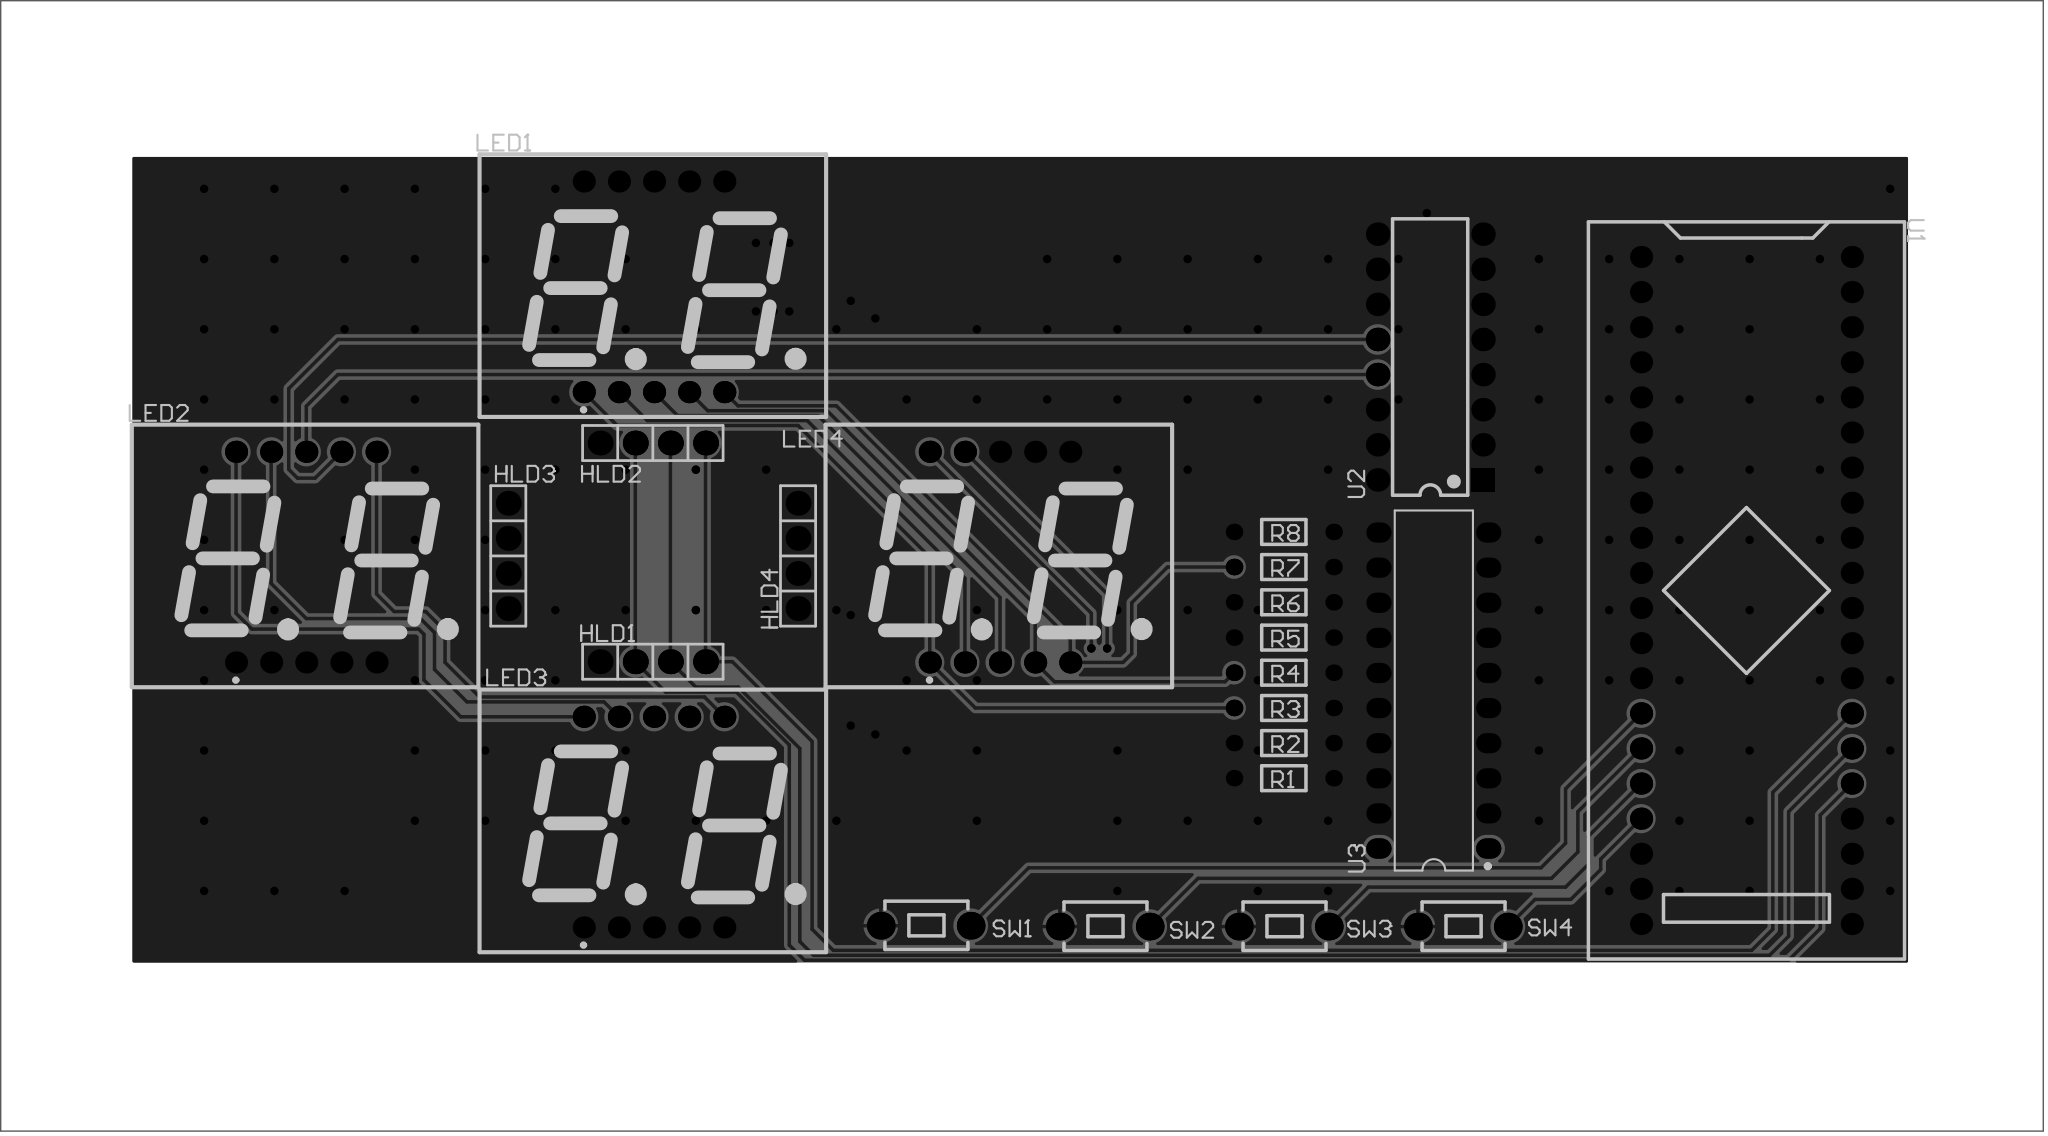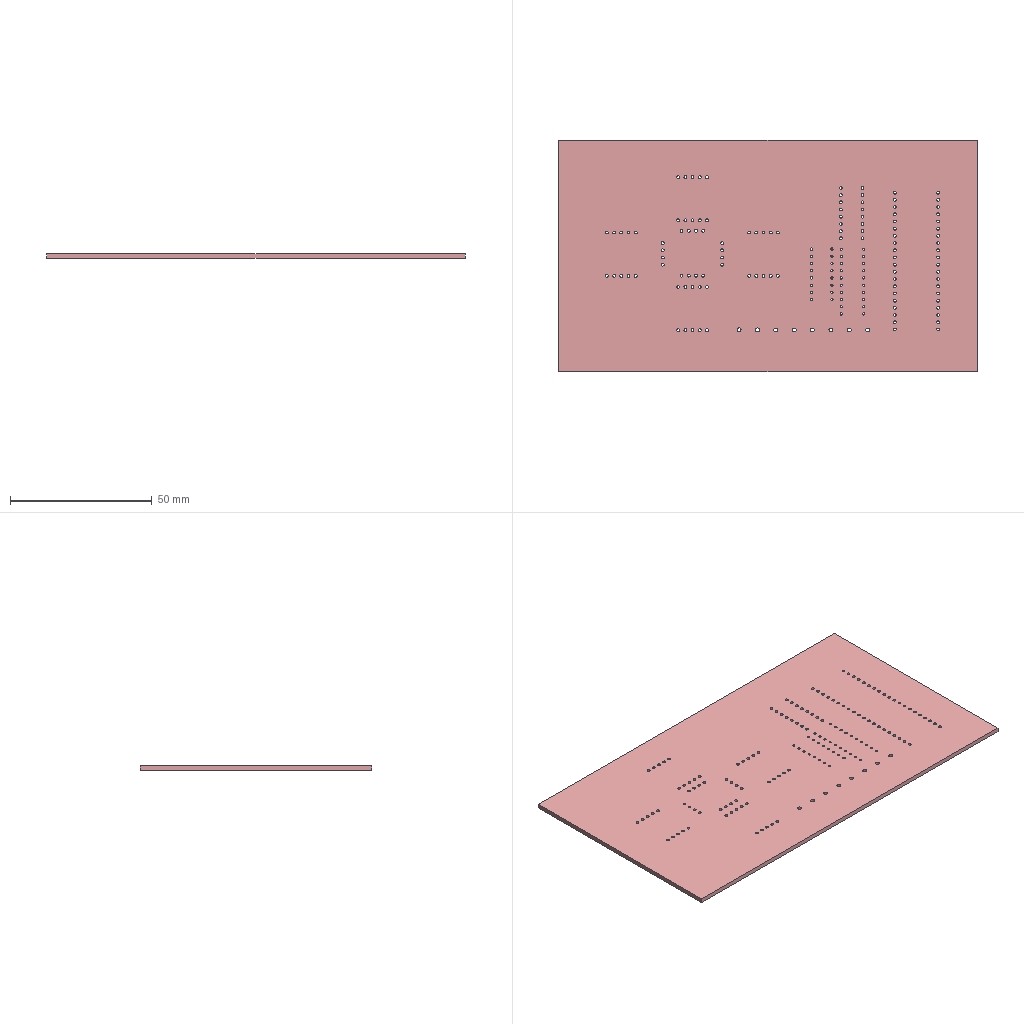Circuit board layout | Altium Designer | box 147.7 x 81.8 x 1.6 mm
Layer stack:
# Altium Designer layer stack of  (unit mm; dielectric type: 0 none, 1 core, 2 prepreg, 3 surface material)
index,name,kind,layer,copper_thickness_mm,dielectric_type,dielectric_thickness_mm,dielectric_material,dielectric_constant
0,Top Paste Mask Layer,other,,,,,,
1,Top Silkscreen Layer,other,,,,,,
2,Top Solder Mask Layer,dielectric,,,3,0.01,,3.3
3,Top Layer,copper,Top Layer,0.035,,,,
4,Dielectric1,dielectric,,,3,1.51,FR4,4.5
5,Bottom Layer,copper,Bottom Layer,0.035,,,,
6,Bottom Solder Mask Layer,dielectric,,,3,0.01,,3.3
7,Bottom Silkscreen Layer,other,,,,,,
8,Bottom Paste Mask Layer,other,,,,,,
# drill layer pairs: low layer,high layer
drill_pair,Top Layer,Bottom Layer
Part placement:
Designator,Comment,Layer,Footprint,Center-X(mm),Center-Y(mm),Rotation
HLD1,,TopLayer,SIP-04,117.007,103.813,0
HLD2,,TopLayer,SIP-04,117.007,119.634,0
HLD3,,TopLayer,SIP-04,106.553,111.465,90
HLD4,,TopLayer,SIP-04,127.508,111.465,90
LED1,SLR0562FW2A3BY-3.5,TopLayer,LED-SEG-TH_10P-L25.0-W19.0-P2.54-S15.24-BL,117.094,130.937,0
LED2,SLR0562FW2A3BY-3.5,TopLayer,LED-SEG-TH_10P-L25.0-W19.0-P2.54-S15.24-BL,91.948,111.379,0
LED3,SLR0562FW2A3BY-3.5,TopLayer,LED-SEG-TH_10P-L25.0-W19.0-P2.54-S15.24-BL,117.094,92.207,0
LED4,SLR0562FW2A3BY-3.5,TopLayer,LED-SEG-TH_10P-L25.0-W19.0-P2.54-S15.24-BL,142.113,111.379,0
R1,100R,TopLayer,Res_1/8W,162.634,95.385,180
R2,100R,TopLayer,Res_1/8W,162.634,97.925,180
R3,100R,TopLayer,Res_1/8W,162.634,100.465,180
R4,100R,TopLayer,Res_1/8W,162.634,103.017,180
R5,100R,TopLayer,Res_1/8W,162.634,105.557,180
R6,100R,TopLayer,Res_1/8W,162.634,108.109,180
R7,100R,TopLayer,Res_1/8W,162.634,110.662,180
R8,100R,TopLayer,Res_1/8W,162.634,113.202,180
SW1,,TopLayer,Key_TH_3.5x6x4.3,136.741,84.709,180
SW2,,TopLayer,Key_TH_3.5x6x4.3,149.688,84.647,180
SW3,,TopLayer,Key_TH_3.5x6x4.3,162.635,84.647,180
SW4,,TopLayer,Key_TH_3.5x6x4.3,175.581,84.647,180
U1,STM32F103C8T6-Card,TopLayer,CONN-TH_L53.3-W22.9_STM32F103C8T6-CARD,196.088,108.966,270
U2,SN74HC138NE4,TopLayer,PDIP-16_L19.7-W6.6-P2.54-LS7.6-BL,173.228,125.857,90
U3,SN74HC245N3,TopLayer,PDIP-20_L25.9-W6.6-P2.54-LS7.9-BL,173.482,101.727,90
Pad and via stacks:
# Altium Designer via and pad stacks of  (unit mm). Each distinct definition once, with the count of objects using it.
# via: kind,start_layer,end_layer,hole_mm,diameter_mm,mode(0 simple;1 top-mid-bottom;2 full stack),diameter_per_layer,count,example_net
# pad: kind,layer,hole_mm,hole_type(0 round;1 square;2 slot),plating,top_size,top_shape(1 round;2 rect;3 octagon;9 rounded rect),mid_size,bottom_size,mode,footprint,size_per_layer,count,example
pad,Multi-Layer,1,0,plated,1.8x1.8,1,1.8x1.8,1.8x1.8,0,SIP-04,,16,HLD1.4
pad,Multi-Layer,1,0,plated,1.6x1.6,1,1.6x1.6,1.6x1.6,0,LED-SEG-TH_10P-L25.0-W19.0-P2.54-S15.24-BL,,40,LED1.4
pad,Multi-Layer,0.8001,0,plated,1.199x1.199,1,1.199x1.199,1.199x1.199,0,Res_1/8W,,16,R1.1
pad,Multi-Layer,1.399,0,plated,1.999x1.999,1,1.999x1.999,1.999x1.999,0,Key_TH_3.5x6x4.3,,8,SW1.A
pad,Multi-Layer,1,0,plated,1.6x1.6,1,1.6x1.6,1.6x1.6,0,CONN-TH_L53.3-W22.9_STM32F103C8T6-CARD,,40,U1.1
pad,Multi-Layer,1,0,plated,1.7x1.7,2,1.7x1.7,1.7x1.7,0,PDIP-16_L19.7-W6.6-P2.54-LS7.6-BL,,1,U2.1
pad,Multi-Layer,1,0,plated,1.7x1.7,1,1.7x1.7,1.7x1.7,0,PDIP-16_L19.7-W6.6-P2.54-LS7.6-BL,,15,U2.2
pad,Multi-Layer,0.8,0,plated,1.462x1.827,1,1.462x1.827,1.462x1.827,0,PDIP-20_L25.9-W6.6-P2.54-LS7.9-BL,,20,U3.1
via,Top Layer,Bottom Layer,0.3048,0.61,0,,174,LED8
Copper pours:
name,layer,net,type(0 solid;1 hatched;2 none)
Top Layer-GND,Top Layer,GND,0
Bottom Layer-GND,Bottom Layer,GND,0